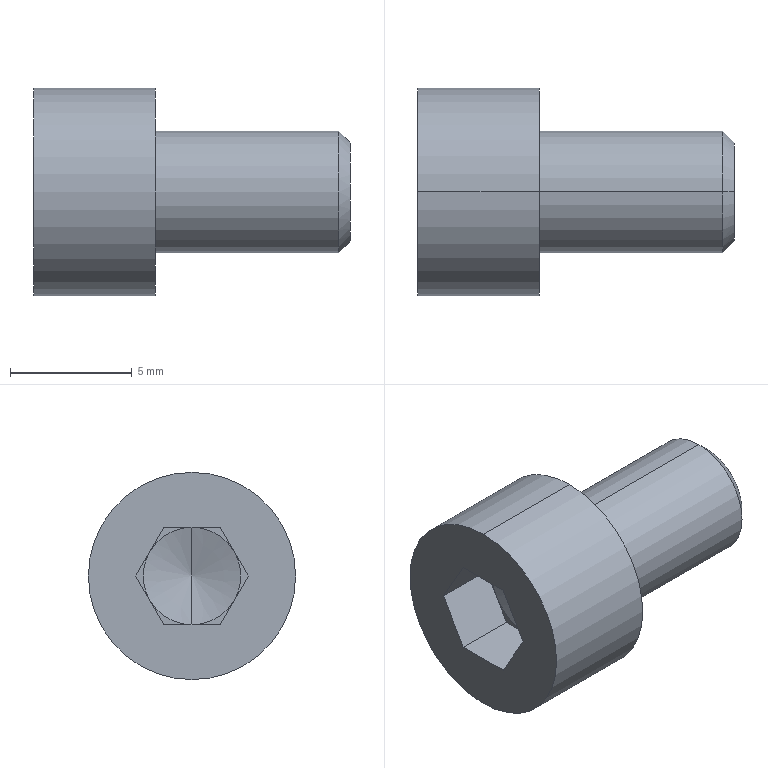Part | SolidWorks | features BaseBody 1 | 1 solid | 23 faces | box 13 x 8.5 x 8.5 mm | volume 402.153 mm3 | plane 15 | cylinder 4 | cone 4 | commonest cylinder face diameters 5 x2 8.5 x2
STEP:
#1=CARTESIAN_POINT('',(-5.,0.,-4.25));
#2=VERTEX_POINT('',#1);
#3=CARTESIAN_POINT('',(-5.,0.,4.25));
#4=VERTEX_POINT('',#3);
#5=CARTESIAN_POINT('',(-5.,0.,0.));
#6=DIRECTION('',(1.,0.,0.));
#7=DIRECTION('',(0.,0.,-1.));
#8=AXIS2_PLACEMENT_3D('',#5,#6,#7);
#9=CIRCLE('',#8,4.25);
#10=EDGE_CURVE('',#2,#4,#9,.T.);
#11=ORIENTED_EDGE('',*,*,#10,.T.);
#12=CARTESIAN_POINT('',(0.,0.,4.25));
#13=VERTEX_POINT('',#12);
#14=CARTESIAN_POINT('',(-2.5,0.,4.25));
#15=DIRECTION('',(1.,0.,0.));
#16=VECTOR('',#15,1000.);
#17=LINE('',#14,#16);
#18=EDGE_CURVE('',#4,#13,#17,.T.);
#19=ORIENTED_EDGE('',*,*,#18,.T.);
#20=CARTESIAN_POINT('',(0.,0.,-4.25));
#21=VERTEX_POINT('',#20);
#22=CARTESIAN_POINT('',(0.,0.,0.));
#23=DIRECTION('',(-1.,0.,0.));
#24=DIRECTION('',(0.,0.,-1.));
#25=AXIS2_PLACEMENT_3D('',#22,#23,#24);
#26=CIRCLE('',#25,4.25);
#27=EDGE_CURVE('',#13,#21,#26,.T.);
#28=ORIENTED_EDGE('',*,*,#27,.T.);
#29=CARTESIAN_POINT('',(-2.5,0.,-4.25));
#30=DIRECTION('',(1.,0.,0.));
#31=VECTOR('',#30,1000.);
#32=LINE('',#29,#31);
#33=EDGE_CURVE('',#2,#21,#32,.T.);
#34=ORIENTED_EDGE('',*,*,#33,.F.);
#35=EDGE_LOOP('',(#11,#19,#28,#34));
#36=FACE_OUTER_BOUND('',#35,.T.);
#37=CARTESIAN_POINT('',(-2.5,0.,0.));
#38=DIRECTION('',(1.,0.,0.));
#39=DIRECTION('',(0.,0.,-1.));
#40=AXIS2_PLACEMENT_3D('',#37,#38,#39);
#41=CYLINDRICAL_SURFACE('',#40,4.25);
#42=ADVANCED_FACE('',(#36),#41,.T.);
#43=CARTESIAN_POINT('',(0.,0.,2.5));
#44=VERTEX_POINT('',#43);
#45=CARTESIAN_POINT('',(0.,0.,-2.5));
#46=VERTEX_POINT('',#45);
#47=CARTESIAN_POINT('',(0.,0.,0.));
#48=DIRECTION('',(-1.,0.,0.));
#49=DIRECTION('',(0.,0.,-1.));
#50=AXIS2_PLACEMENT_3D('',#47,#48,#49);
#51=CIRCLE('',#50,2.5);
#52=EDGE_CURVE('',#44,#46,#51,.T.);
#53=ORIENTED_EDGE('',*,*,#52,.F.);
#54=CARTESIAN_POINT('',(7.51,0.,2.5));
#55=VERTEX_POINT('',#54);
#56=CARTESIAN_POINT('',(3.755,0.,2.5));
#57=DIRECTION('',(1.,0.,0.));
#58=VECTOR('',#57,1000.);
#59=LINE('',#56,#58);
#60=EDGE_CURVE('',#44,#55,#59,.T.);
#61=ORIENTED_EDGE('',*,*,#60,.T.);
#62=CARTESIAN_POINT('',(7.51,0.,-2.5));
#63=VERTEX_POINT('',#62);
#64=CARTESIAN_POINT('',(7.51,0.,0.));
#65=DIRECTION('',(-1.,0.,0.));
#66=DIRECTION('',(0.,0.,-1.));
#67=AXIS2_PLACEMENT_3D('',#64,#65,#66);
#68=CIRCLE('',#67,2.5);
#69=EDGE_CURVE('',#55,#63,#68,.T.);
#70=ORIENTED_EDGE('',*,*,#69,.T.);
#71=CARTESIAN_POINT('',(3.755,0.,-2.5));
#72=DIRECTION('',(1.,0.,0.));
#73=VECTOR('',#72,1000.);
#74=LINE('',#71,#73);
#75=EDGE_CURVE('',#46,#63,#74,.T.);
#76=ORIENTED_EDGE('',*,*,#75,.F.);
#77=EDGE_LOOP('',(#53,#61,#70,#76));
#78=FACE_OUTER_BOUND('',#77,.T.);
#79=CARTESIAN_POINT('',(3.755,0.,0.));
#80=DIRECTION('',(1.,0.,0.));
#81=DIRECTION('',(0.,0.,-1.));
#82=AXIS2_PLACEMENT_3D('',#79,#80,#81);
#83=CYLINDRICAL_SURFACE('',#82,2.5);
#84=ADVANCED_FACE('',(#78),#83,.T.);
#85=CARTESIAN_POINT('',(8.,0.,2.009));
#86=VERTEX_POINT('',#85);
#87=CARTESIAN_POINT('',(8.,0.,-2.009));
#88=VERTEX_POINT('',#87);
#89=CARTESIAN_POINT('',(8.,0.,0.));
#90=DIRECTION('',(-1.,0.,0.));
#91=DIRECTION('',(0.,0.,1.));
#92=AXIS2_PLACEMENT_3D('',#89,#90,#91);
#93=CIRCLE('',#92,2.009);
#94=EDGE_CURVE('',#86,#88,#93,.T.);
#95=ORIENTED_EDGE('',*,*,#94,.T.);
#96=CARTESIAN_POINT('',(7.51,0.,-2.5));
#97=DIRECTION('',(-0.7071,0.,-0.7071));
#98=VECTOR('',#97,1000.);
#99=LINE('',#96,#98);
#100=EDGE_CURVE('',#88,#63,#99,.T.);
#101=ORIENTED_EDGE('',*,*,#100,.T.);
#102=ORIENTED_EDGE('',*,*,#69,.F.);
#103=CARTESIAN_POINT('',(7.51,0.,2.5));
#104=DIRECTION('',(-0.7071,0.,0.7071));
#105=VECTOR('',#104,1000.);
#106=LINE('',#103,#105);
#107=EDGE_CURVE('',#86,#55,#106,.T.);
#108=ORIENTED_EDGE('',*,*,#107,.F.);
#109=EDGE_LOOP('',(#95,#101,#102,#108));
#110=FACE_OUTER_BOUND('',#109,.T.);
#111=CARTESIAN_POINT('',(7.51,0.,0.));
#112=DIRECTION('',(-1.,0.,0.));
#113=DIRECTION('',(0.,0.,1.));
#114=AXIS2_PLACEMENT_3D('',#111,#112,#113);
#115=CONICAL_SURFACE('',#114,2.5,0.7854);
#116=ADVANCED_FACE('',(#110),#115,.T.);
#117=CARTESIAN_POINT('',(-1.964,0.000000001,0.));
#118=VERTEX_POINT('',#117);
#119=CARTESIAN_POINT('',(-2.5,0.,2.));
#120=VERTEX_POINT('',#119);
#121=CARTESIAN_POINT('',(-2.5,0.,2.));
#122=DIRECTION('',(-0.2588,0.,0.9659));
#123=VECTOR('',#122,1000.);
#124=LINE('',#121,#123);
#125=EDGE_CURVE('',#118,#120,#124,.T.);
#126=ORIENTED_EDGE('',*,*,#125,.F.);
#127=CARTESIAN_POINT('',(-2.5,0.,-2.));
#128=VERTEX_POINT('',#127);
#129=CARTESIAN_POINT('',(-2.5,0.,-2.));
#130=DIRECTION('',(-0.2588,0.,-0.9659));
#131=VECTOR('',#130,1000.);
#132=LINE('',#129,#131);
#133=EDGE_CURVE('',#118,#128,#132,.T.);
#134=ORIENTED_EDGE('',*,*,#133,.T.);
#135=CARTESIAN_POINT('',(-2.5,-1.732,-1.));
#136=VERTEX_POINT('',#135);
#137=CARTESIAN_POINT('',(-2.5,0.,0.));
#138=DIRECTION('',(1.,0.,0.));
#139=DIRECTION('',(0.,0.,1.));
#140=AXIS2_PLACEMENT_3D('',#137,#138,#139);
#141=CIRCLE('',#140,2.);
#142=EDGE_CURVE('',#136,#128,#141,.T.);
#143=ORIENTED_EDGE('',*,*,#142,.F.);
#144=CARTESIAN_POINT('',(-2.5,-1.732,1.));
#145=VERTEX_POINT('',#144);
#146=CARTESIAN_POINT('',(-2.5,0.,0.));
#147=DIRECTION('',(1.,0.,0.));
#148=DIRECTION('',(0.,0.,1.));
#149=AXIS2_PLACEMENT_3D('',#146,#147,#148);
#150=CIRCLE('',#149,2.);
#151=EDGE_CURVE('',#145,#136,#150,.T.);
#152=ORIENTED_EDGE('',*,*,#151,.F.);
#153=CARTESIAN_POINT('',(-2.5,0.,0.));
#154=DIRECTION('',(-1.,0.,0.));
#155=DIRECTION('',(0.,0.,1.));
#156=AXIS2_PLACEMENT_3D('',#153,#154,#155);
#157=CIRCLE('',#156,2.);
#158=EDGE_CURVE('',#145,#120,#157,.T.);
#159=ORIENTED_EDGE('',*,*,#158,.T.);
#160=EDGE_LOOP('',(#126,#134,#143,#152,#159));
#161=FACE_OUTER_BOUND('',#160,.T.);
#162=CARTESIAN_POINT('',(-2.5,0.,0.));
#163=DIRECTION('',(-1.,0.,0.));
#164=DIRECTION('',(0.,0.,1.));
#165=AXIS2_PLACEMENT_3D('',#162,#163,#164);
#166=CONICAL_SURFACE('',#165,2.,1.309);
#167=ADVANCED_FACE('',(#161),#166,.F.);
#168=ORIENTED_EDGE('',*,*,#18,.F.);
#169=CARTESIAN_POINT('',(-5.,0.,0.));
#170=DIRECTION('',(1.,0.,0.));
#171=DIRECTION('',(0.,0.,-1.));
#172=AXIS2_PLACEMENT_3D('',#169,#170,#171);
#173=CIRCLE('',#172,4.25);
#174=EDGE_CURVE('',#4,#2,#173,.T.);
#175=ORIENTED_EDGE('',*,*,#174,.T.);
#176=ORIENTED_EDGE('',*,*,#33,.T.);
#177=CARTESIAN_POINT('',(0.,0.,0.));
#178=DIRECTION('',(-1.,0.,0.));
#179=DIRECTION('',(0.,0.,-1.));
#180=AXIS2_PLACEMENT_3D('',#177,#178,#179);
#181=CIRCLE('',#180,4.25);
#182=EDGE_CURVE('',#21,#13,#181,.T.);
#183=ORIENTED_EDGE('',*,*,#182,.T.);
#184=EDGE_LOOP('',(#168,#175,#176,#183));
#185=FACE_OUTER_BOUND('',#184,.T.);
#186=CARTESIAN_POINT('',(-2.5,0.,0.));
#187=DIRECTION('',(1.,0.,0.));
#188=DIRECTION('',(0.,0.,-1.));
#189=AXIS2_PLACEMENT_3D('',#186,#187,#188);
#190=CYLINDRICAL_SURFACE('',#189,4.25);
#191=ADVANCED_FACE('',(#185),#190,.T.);
#192=ORIENTED_EDGE('',*,*,#10,.F.);
#193=ORIENTED_EDGE('',*,*,#174,.F.);
#194=EDGE_LOOP('',(#192,#193));
#195=FACE_OUTER_BOUND('',#194,.T.);
#196=CARTESIAN_POINT('',(-5.,1.155,-2.));
#197=VERTEX_POINT('',#196);
#198=CARTESIAN_POINT('',(-5.,2.309,0.));
#199=VERTEX_POINT('',#198);
#200=CARTESIAN_POINT('',(-5.,1.155,-2.));
#201=DIRECTION('',(0.,0.5,0.866));
#202=VECTOR('',#201,1000.);
#203=LINE('',#200,#202);
#204=EDGE_CURVE('',#197,#199,#203,.T.);
#205=ORIENTED_EDGE('',*,*,#204,.T.);
#206=CARTESIAN_POINT('',(-5.,1.155,2.));
#207=VERTEX_POINT('',#206);
#208=CARTESIAN_POINT('',(-5.,2.309,0.));
#209=DIRECTION('',(0.,-0.5,0.866));
#210=VECTOR('',#209,1000.);
#211=LINE('',#208,#210);
#212=EDGE_CURVE('',#199,#207,#211,.T.);
#213=ORIENTED_EDGE('',*,*,#212,.T.);
#214=CARTESIAN_POINT('',(-5.,-1.155,2.));
#215=VERTEX_POINT('',#214);
#216=CARTESIAN_POINT('',(-5.,2.125,2.));
#217=DIRECTION('',(0.,-1.,0.));
#218=VECTOR('',#217,1000.);
#219=LINE('',#216,#218);
#220=EDGE_CURVE('',#207,#215,#219,.T.);
#221=ORIENTED_EDGE('',*,*,#220,.T.);
#222=CARTESIAN_POINT('',(-5.,-2.309,0.));
#223=VERTEX_POINT('',#222);
#224=CARTESIAN_POINT('',(-5.,-1.155,2.));
#225=DIRECTION('',(0.,-0.5,-0.866));
#226=VECTOR('',#225,1000.);
#227=LINE('',#224,#226);
#228=EDGE_CURVE('',#215,#223,#227,.T.);
#229=ORIENTED_EDGE('',*,*,#228,.T.);
#230=CARTESIAN_POINT('',(-5.,-1.155,-2.));
#231=VERTEX_POINT('',#230);
#232=CARTESIAN_POINT('',(-5.,-2.309,0.));
#233=DIRECTION('',(0.,0.5,-0.866));
#234=VECTOR('',#233,1000.);
#235=LINE('',#232,#234);
#236=EDGE_CURVE('',#223,#231,#235,.T.);
#237=ORIENTED_EDGE('',*,*,#236,.T.);
#238=CARTESIAN_POINT('',(-5.,2.125,-2.));
#239=DIRECTION('',(0.,1.,0.));
#240=VECTOR('',#239,1000.);
#241=LINE('',#238,#240);
#242=EDGE_CURVE('',#231,#197,#241,.T.);
#243=ORIENTED_EDGE('',*,*,#242,.T.);
#244=EDGE_LOOP('',(#205,#213,#221,#229,#237,#243));
#245=FACE_BOUND('',#244,.T.);
#246=CARTESIAN_POINT('',(-5.,2.125,0.));
#247=DIRECTION('',(-1.,0.,0.));
#248=DIRECTION('',(0.,0.,1.));
#249=AXIS2_PLACEMENT_3D('',#246,#247,#248);
#250=PLANE('',#249);
#251=ADVANCED_FACE('',(#195,#245),#250,.T.);
#252=CARTESIAN_POINT('',(0.,0.,0.));
#253=DIRECTION('',(-1.,0.,0.));
#254=DIRECTION('',(0.,0.,-1.));
#255=AXIS2_PLACEMENT_3D('',#252,#253,#254);
#256=CIRCLE('',#255,2.5);
#257=EDGE_CURVE('',#46,#44,#256,.T.);
#258=ORIENTED_EDGE('',*,*,#257,.T.);
#259=ORIENTED_EDGE('',*,*,#52,.T.);
#260=EDGE_LOOP('',(#258,#259));
#261=FACE_BOUND('',#260,.T.);
#262=ORIENTED_EDGE('',*,*,#182,.F.);
#263=ORIENTED_EDGE('',*,*,#27,.F.);
#264=EDGE_LOOP('',(#262,#263));
#265=FACE_OUTER_BOUND('',#264,.T.);
#266=CARTESIAN_POINT('',(0.,3.375,0.));
#267=DIRECTION('',(1.,0.,0.));
#268=DIRECTION('',(0.,0.,-1.));
#269=AXIS2_PLACEMENT_3D('',#266,#267,#268);
#270=PLANE('',#269);
#271=ADVANCED_FACE('',(#261,#265),#270,.T.);
#272=CARTESIAN_POINT('',(-2.5,2.309,0.));
#273=VERTEX_POINT('',#272);
#274=CARTESIAN_POINT('',(-5.,2.309,0.));
#275=DIRECTION('',(-1.,0.,0.));
#276=VECTOR('',#275,1000.);
#277=LINE('',#274,#276);
#278=EDGE_CURVE('',#273,#199,#277,.T.);
#279=ORIENTED_EDGE('',*,*,#278,.F.);
#280=CARTESIAN_POINT('',(-2.5,1.732,1.));
#281=VERTEX_POINT('',#280);
#282=CARTESIAN_POINT('',(-2.5,1.155,2.));
#283=DIRECTION('',(0.,0.5,-0.866));
#284=VECTOR('',#283,1000.);
#285=LINE('',#282,#284);
#286=EDGE_CURVE('',#281,#273,#285,.T.);
#287=ORIENTED_EDGE('',*,*,#286,.F.);
#288=CARTESIAN_POINT('',(-2.5,1.155,2.));
#289=VERTEX_POINT('',#288);
#290=CARTESIAN_POINT('',(-2.5,1.732,1.));
#291=DIRECTION('',(0.,-0.5,0.866));
#292=VECTOR('',#291,1000.);
#293=LINE('',#290,#292);
#294=EDGE_CURVE('',#281,#289,#293,.T.);
#295=ORIENTED_EDGE('',*,*,#294,.T.);
#296=CARTESIAN_POINT('',(-5.,1.155,2.));
#297=DIRECTION('',(1.,0.,0.));
#298=VECTOR('',#297,1000.);
#299=LINE('',#296,#298);
#300=EDGE_CURVE('',#207,#289,#299,.T.);
#301=ORIENTED_EDGE('',*,*,#300,.F.);
#302=ORIENTED_EDGE('',*,*,#212,.F.);
#303=EDGE_LOOP('',(#279,#287,#295,#301,#302));
#304=FACE_OUTER_BOUND('',#303,.T.);
#305=CARTESIAN_POINT('',(-5.,1.155,2.));
#306=DIRECTION('',(0.,0.866,0.5));
#307=DIRECTION('',(0.,-0.5,0.866));
#308=AXIS2_PLACEMENT_3D('',#305,#306,#307);
#309=PLANE('',#308);
#310=ADVANCED_FACE('',(#304),#309,.F.);
#311=CARTESIAN_POINT('',(-2.5,1.155,-2.));
#312=VERTEX_POINT('',#311);
#313=CARTESIAN_POINT('',(-5.,1.155,-2.));
#314=DIRECTION('',(-1.,0.,0.));
#315=VECTOR('',#314,1000.);
#316=LINE('',#313,#315);
#317=EDGE_CURVE('',#312,#197,#316,.T.);
#318=ORIENTED_EDGE('',*,*,#317,.F.);
#319=CARTESIAN_POINT('',(-2.5,1.732,-1.));
#320=VERTEX_POINT('',#319);
#321=CARTESIAN_POINT('',(-2.5,1.155,-2.));
#322=DIRECTION('',(0.,0.5,0.866));
#323=VECTOR('',#322,1000.);
#324=LINE('',#321,#323);
#325=EDGE_CURVE('',#312,#320,#324,.T.);
#326=ORIENTED_EDGE('',*,*,#325,.T.);
#327=CARTESIAN_POINT('',(-2.5,2.309,0.));
#328=DIRECTION('',(0.,-0.5,-0.866));
#329=VECTOR('',#328,1000.);
#330=LINE('',#327,#329);
#331=EDGE_CURVE('',#273,#320,#330,.T.);
#332=ORIENTED_EDGE('',*,*,#331,.F.);
#333=ORIENTED_EDGE('',*,*,#278,.T.);
#334=ORIENTED_EDGE('',*,*,#204,.F.);
#335=EDGE_LOOP('',(#318,#326,#332,#333,#334));
#336=FACE_OUTER_BOUND('',#335,.T.);
#337=CARTESIAN_POINT('',(-5.,2.309,0.));
#338=DIRECTION('',(0.,0.866,-0.5));
#339=DIRECTION('',(0.,0.5,0.866));
#340=AXIS2_PLACEMENT_3D('',#337,#338,#339);
#341=PLANE('',#340);
#342=ADVANCED_FACE('',(#336),#341,.F.);
#343=CARTESIAN_POINT('',(-2.5,-1.155,-2.));
#344=VERTEX_POINT('',#343);
#345=CARTESIAN_POINT('',(-5.,-1.155,-2.));
#346=DIRECTION('',(-1.,0.,0.));
#347=VECTOR('',#346,1000.);
#348=LINE('',#345,#347);
#349=EDGE_CURVE('',#344,#231,#348,.T.);
#350=ORIENTED_EDGE('',*,*,#349,.F.);
#351=CARTESIAN_POINT('',(-2.5,0.,-2.));
#352=DIRECTION('',(0.,1.,0.));
#353=VECTOR('',#352,1000.);
#354=LINE('',#351,#353);
#355=EDGE_CURVE('',#344,#128,#354,.T.);
#356=ORIENTED_EDGE('',*,*,#355,.T.);
#357=CARTESIAN_POINT('',(-2.5,0.,-2.));
#358=DIRECTION('',(0.,1.,0.));
#359=VECTOR('',#358,1000.);
#360=LINE('',#357,#359);
#361=EDGE_CURVE('',#128,#312,#360,.T.);
#362=ORIENTED_EDGE('',*,*,#361,.T.);
#363=ORIENTED_EDGE('',*,*,#317,.T.);
#364=ORIENTED_EDGE('',*,*,#242,.F.);
#365=EDGE_LOOP('',(#350,#356,#362,#363,#364));
#366=FACE_OUTER_BOUND('',#365,.T.);
#367=CARTESIAN_POINT('',(-5.,1.155,-2.));
#368=DIRECTION('',(0.,0.,-1.));
#369=DIRECTION('',(-1.,0.,0.));
#370=AXIS2_PLACEMENT_3D('',#367,#368,#369);
#371=PLANE('',#370);
#372=ADVANCED_FACE('',(#366),#371,.F.);
#373=CARTESIAN_POINT('',(-2.5,-2.309,0.));
#374=VERTEX_POINT('',#373);
#375=CARTESIAN_POINT('',(-5.,-2.309,0.));
#376=DIRECTION('',(-1.,0.,0.));
#377=VECTOR('',#376,1000.);
#378=LINE('',#375,#377);
#379=EDGE_CURVE('',#374,#223,#378,.T.);
#380=ORIENTED_EDGE('',*,*,#379,.F.);
#381=CARTESIAN_POINT('',(-2.5,-1.155,-2.));
#382=DIRECTION('',(0.,-0.5,0.866));
#383=VECTOR('',#382,1000.);
#384=LINE('',#381,#383);
#385=EDGE_CURVE('',#136,#374,#384,.T.);
#386=ORIENTED_EDGE('',*,*,#385,.F.);
#387=CARTESIAN_POINT('',(-2.5,-1.732,-1.));
#388=DIRECTION('',(0.,0.5,-0.866));
#389=VECTOR('',#388,1000.);
#390=LINE('',#387,#389);
#391=EDGE_CURVE('',#136,#344,#390,.T.);
#392=ORIENTED_EDGE('',*,*,#391,.T.);
#393=ORIENTED_EDGE('',*,*,#349,.T.);
#394=ORIENTED_EDGE('',*,*,#236,.F.);
#395=EDGE_LOOP('',(#380,#386,#392,#393,#394));
#396=FACE_OUTER_BOUND('',#395,.T.);
#397=CARTESIAN_POINT('',(-5.,-1.155,-2.));
#398=DIRECTION('',(0.,-0.866,-0.5));
#399=DIRECTION('',(0.,0.5,-0.866));
#400=AXIS2_PLACEMENT_3D('',#397,#398,#399);
#401=PLANE('',#400);
#402=ADVANCED_FACE('',(#396),#401,.F.);
#403=CARTESIAN_POINT('',(-2.5,-1.155,2.));
#404=VERTEX_POINT('',#403);
#405=CARTESIAN_POINT('',(-5.,-1.155,2.));
#406=DIRECTION('',(-1.,0.,0.));
#407=VECTOR('',#406,1000.);
#408=LINE('',#405,#407);
#409=EDGE_CURVE('',#404,#215,#408,.T.);
#410=ORIENTED_EDGE('',*,*,#409,.F.);
#411=CARTESIAN_POINT('',(-2.5,-2.309,0.));
#412=DIRECTION('',(0.,0.5,0.866));
#413=VECTOR('',#412,1000.);
#414=LINE('',#411,#413);
#415=EDGE_CURVE('',#145,#404,#414,.T.);
#416=ORIENTED_EDGE('',*,*,#415,.F.);
#417=CARTESIAN_POINT('',(-2.5,-2.309,0.));
#418=DIRECTION('',(0.,0.5,0.866));
#419=VECTOR('',#418,1000.);
#420=LINE('',#417,#419);
#421=EDGE_CURVE('',#374,#145,#420,.T.);
#422=ORIENTED_EDGE('',*,*,#421,.F.);
#423=ORIENTED_EDGE('',*,*,#379,.T.);
#424=ORIENTED_EDGE('',*,*,#228,.F.);
#425=EDGE_LOOP('',(#410,#416,#422,#423,#424));
#426=FACE_OUTER_BOUND('',#425,.T.);
#427=CARTESIAN_POINT('',(-5.,-2.309,0.));
#428=DIRECTION('',(0.,-0.866,0.5));
#429=DIRECTION('',(0.,-0.5,-0.866));
#430=AXIS2_PLACEMENT_3D('',#427,#428,#429);
#431=PLANE('',#430);
#432=ADVANCED_FACE('',(#426),#431,.F.);
#433=ORIENTED_EDGE('',*,*,#300,.T.);
#434=CARTESIAN_POINT('',(-2.5,0.,2.));
#435=DIRECTION('',(0.,-1.,0.));
#436=VECTOR('',#435,1000.);
#437=LINE('',#434,#436);
#438=EDGE_CURVE('',#289,#120,#437,.T.);
#439=ORIENTED_EDGE('',*,*,#438,.T.);
#440=CARTESIAN_POINT('',(-2.5,-1.155,2.));
#441=DIRECTION('',(0.,1.,0.));
#442=VECTOR('',#441,1000.);
#443=LINE('',#440,#442);
#444=EDGE_CURVE('',#404,#120,#443,.T.);
#445=ORIENTED_EDGE('',*,*,#444,.F.);
#446=ORIENTED_EDGE('',*,*,#409,.T.);
#447=ORIENTED_EDGE('',*,*,#220,.F.);
#448=EDGE_LOOP('',(#433,#439,#445,#446,#447));
#449=FACE_OUTER_BOUND('',#448,.T.);
#450=CARTESIAN_POINT('',(-5.,-1.155,2.));
#451=DIRECTION('',(0.,0.,1.));
#452=DIRECTION('',(1.,0.,0.));
#453=AXIS2_PLACEMENT_3D('',#450,#451,#452);
#454=PLANE('',#453);
#455=ADVANCED_FACE('',(#449),#454,.F.);
#456=ORIENTED_EDGE('',*,*,#60,.F.);
#457=ORIENTED_EDGE('',*,*,#257,.F.);
#458=ORIENTED_EDGE('',*,*,#75,.T.);
#459=CARTESIAN_POINT('',(7.51,0.,0.));
#460=DIRECTION('',(-1.,0.,0.));
#461=DIRECTION('',(0.,0.,-1.));
#462=AXIS2_PLACEMENT_3D('',#459,#460,#461);
#463=CIRCLE('',#462,2.5);
#464=EDGE_CURVE('',#63,#55,#463,.T.);
#465=ORIENTED_EDGE('',*,*,#464,.T.);
#466=EDGE_LOOP('',(#456,#457,#458,#465));
#467=FACE_OUTER_BOUND('',#466,.T.);
#468=CARTESIAN_POINT('',(3.755,0.,0.));
#469=DIRECTION('',(1.,0.,0.));
#470=DIRECTION('',(0.,0.,-1.));
#471=AXIS2_PLACEMENT_3D('',#468,#469,#470);
#472=CYLINDRICAL_SURFACE('',#471,2.5);
#473=ADVANCED_FACE('',(#467),#472,.T.);
#474=ORIENTED_EDGE('',*,*,#286,.T.);
#475=ORIENTED_EDGE('',*,*,#331,.T.);
#476=CARTESIAN_POINT('',(-2.5,0.,0.));
#477=DIRECTION('',(1.,0.,0.));
#478=DIRECTION('',(0.,0.,1.));
#479=AXIS2_PLACEMENT_3D('',#476,#477,#478);
#480=CIRCLE('',#479,2.);
#481=EDGE_CURVE('',#320,#281,#480,.T.);
#482=ORIENTED_EDGE('',*,*,#481,.T.);
#483=EDGE_LOOP('',(#474,#475,#482));
#484=FACE_OUTER_BOUND('',#483,.T.);
#485=CARTESIAN_POINT('',(-2.5,0.,0.));
#486=DIRECTION('',(1.,0.,0.));
#487=DIRECTION('',(0.,0.,-1.));
#488=AXIS2_PLACEMENT_3D('',#485,#486,#487);
#489=PLANE('',#488);
#490=ADVANCED_FACE('',(#484),#489,.F.);
#491=ORIENTED_EDGE('',*,*,#385,.T.);
#492=ORIENTED_EDGE('',*,*,#421,.T.);
#493=ORIENTED_EDGE('',*,*,#151,.T.);
#494=EDGE_LOOP('',(#491,#492,#493));
#495=FACE_OUTER_BOUND('',#494,.T.);
#496=CARTESIAN_POINT('',(-2.5,0.,0.));
#497=DIRECTION('',(1.,0.,0.));
#498=DIRECTION('',(0.,0.,-1.));
#499=AXIS2_PLACEMENT_3D('',#496,#497,#498);
#500=PLANE('',#499);
#501=ADVANCED_FACE('',(#495),#500,.F.);
#502=ORIENTED_EDGE('',*,*,#415,.T.);
#503=ORIENTED_EDGE('',*,*,#444,.T.);
#504=ORIENTED_EDGE('',*,*,#158,.F.);
#505=EDGE_LOOP('',(#502,#503,#504));
#506=FACE_OUTER_BOUND('',#505,.T.);
#507=CARTESIAN_POINT('',(-2.5,0.,0.));
#508=DIRECTION('',(1.,0.,0.));
#509=DIRECTION('',(0.,0.,-1.));
#510=AXIS2_PLACEMENT_3D('',#507,#508,#509);
#511=PLANE('',#510);
#512=ADVANCED_FACE('',(#506),#511,.F.);
#513=ORIENTED_EDGE('',*,*,#100,.F.);
#514=CARTESIAN_POINT('',(8.,0.,0.));
#515=DIRECTION('',(-1.,0.,0.));
#516=DIRECTION('',(0.,0.,1.));
#517=AXIS2_PLACEMENT_3D('',#514,#515,#516);
#518=CIRCLE('',#517,2.009);
#519=EDGE_CURVE('',#88,#86,#518,.T.);
#520=ORIENTED_EDGE('',*,*,#519,.T.);
#521=ORIENTED_EDGE('',*,*,#107,.T.);
#522=ORIENTED_EDGE('',*,*,#464,.F.);
#523=EDGE_LOOP('',(#513,#520,#521,#522));
#524=FACE_OUTER_BOUND('',#523,.T.);
#525=CARTESIAN_POINT('',(7.51,0.,0.));
#526=DIRECTION('',(-1.,0.,0.));
#527=DIRECTION('',(0.,0.,1.));
#528=AXIS2_PLACEMENT_3D('',#525,#526,#527);
#529=CONICAL_SURFACE('',#528,2.5,0.7854);
#530=ADVANCED_FACE('',(#524),#529,.T.);
#531=ORIENTED_EDGE('',*,*,#133,.F.);
#532=ORIENTED_EDGE('',*,*,#125,.T.);
#533=CARTESIAN_POINT('',(-2.5,0.,0.));
#534=DIRECTION('',(1.,0.,0.));
#535=DIRECTION('',(0.,0.,1.));
#536=AXIS2_PLACEMENT_3D('',#533,#534,#535);
#537=CIRCLE('',#536,2.);
#538=EDGE_CURVE('',#281,#120,#537,.T.);
#539=ORIENTED_EDGE('',*,*,#538,.F.);
#540=ORIENTED_EDGE('',*,*,#481,.F.);
#541=CARTESIAN_POINT('',(-2.5,0.,0.));
#542=DIRECTION('',(1.,0.,0.));
#543=DIRECTION('',(0.,0.,1.));
#544=AXIS2_PLACEMENT_3D('',#541,#542,#543);
#545=CIRCLE('',#544,2.);
#546=EDGE_CURVE('',#128,#320,#545,.T.);
#547=ORIENTED_EDGE('',*,*,#546,.F.);
#548=EDGE_LOOP('',(#531,#532,#539,#540,#547));
#549=FACE_OUTER_BOUND('',#548,.T.);
#550=CARTESIAN_POINT('',(-2.5,0.,0.));
#551=DIRECTION('',(-1.,0.,0.));
#552=DIRECTION('',(0.,0.,1.));
#553=AXIS2_PLACEMENT_3D('',#550,#551,#552);
#554=CONICAL_SURFACE('',#553,2.,1.309);
#555=ADVANCED_FACE('',(#549),#554,.F.);
#556=ORIENTED_EDGE('',*,*,#94,.F.);
#557=ORIENTED_EDGE('',*,*,#519,.F.);
#558=EDGE_LOOP('',(#556,#557));
#559=FACE_OUTER_BOUND('',#558,.T.);
#560=CARTESIAN_POINT('',(8.,1.005,0.));
#561=DIRECTION('',(1.,0.,0.));
#562=DIRECTION('',(0.,0.,-1.));
#563=AXIS2_PLACEMENT_3D('',#560,#561,#562);
#564=PLANE('',#563);
#565=ADVANCED_FACE('',(#559),#564,.T.);
#566=ORIENTED_EDGE('',*,*,#438,.F.);
#567=ORIENTED_EDGE('',*,*,#294,.F.);
#568=ORIENTED_EDGE('',*,*,#538,.T.);
#569=EDGE_LOOP('',(#566,#567,#568));
#570=FACE_OUTER_BOUND('',#569,.T.);
#571=CARTESIAN_POINT('',(-2.5,0.,0.));
#572=DIRECTION('',(1.,0.,0.));
#573=DIRECTION('',(0.,0.,-1.));
#574=AXIS2_PLACEMENT_3D('',#571,#572,#573);
#575=PLANE('',#574);
#576=ADVANCED_FACE('',(#570),#575,.F.);
#577=ORIENTED_EDGE('',*,*,#325,.F.);
#578=ORIENTED_EDGE('',*,*,#361,.F.);
#579=ORIENTED_EDGE('',*,*,#546,.T.);
#580=EDGE_LOOP('',(#577,#578,#579));
#581=FACE_OUTER_BOUND('',#580,.T.);
#582=CARTESIAN_POINT('',(-2.5,0.,0.));
#583=DIRECTION('',(1.,0.,0.));
#584=DIRECTION('',(0.,0.,-1.));
#585=AXIS2_PLACEMENT_3D('',#582,#583,#584);
#586=PLANE('',#585);
#587=ADVANCED_FACE('',(#581),#586,.F.);
#588=ORIENTED_EDGE('',*,*,#355,.F.);
#589=ORIENTED_EDGE('',*,*,#391,.F.);
#590=ORIENTED_EDGE('',*,*,#142,.T.);
#591=EDGE_LOOP('',(#588,#589,#590));
#592=FACE_OUTER_BOUND('',#591,.T.);
#593=CARTESIAN_POINT('',(-2.5,0.,0.));
#594=DIRECTION('',(1.,0.,0.));
#595=DIRECTION('',(0.,0.,-1.));
#596=AXIS2_PLACEMENT_3D('',#593,#594,#595);
#597=PLANE('',#596);
#598=ADVANCED_FACE('',(#592),#597,.F.);
#599=CLOSED_SHELL('',(#42,#84,#116,#167,#191,#251,#271,#310,#342,#372,#402,#432,#455,#473,#490,#501,#512,#530,#555,#565,#576,#587,#598));
#600=MANIFOLD_SOLID_BREP('',#599);
#601=CARTESIAN_POINT('',(0.,0.,0.));
#602=DIRECTION('',(0.,0.,1.));
#603=DIRECTION('',(1.,0.,0.));
#604=AXIS2_PLACEMENT_3D('',#601,#602,#603);
#605=(LENGTH_UNIT()NAMED_UNIT(*)SI_UNIT(.MILLI.,.METRE.));
#606=UNCERTAINTY_MEASURE_WITH_UNIT(LENGTH_MEASURE(0.00001),#605,'','');
#607=(NAMED_UNIT(*)PLANE_ANGLE_UNIT()SI_UNIT($,.RADIAN.));
#608=(NAMED_UNIT(*)SI_UNIT($,.STERADIAN.)SOLID_ANGLE_UNIT());
#609=(GEOMETRIC_REPRESENTATION_CONTEXT(3)GLOBAL_UNCERTAINTY_ASSIGNED_CONTEXT((#606))GLOBAL_UNIT_ASSIGNED_CONTEXT((#605,#607,#608))REPRESENTATION_CONTEXT('',''));
#610=ADVANCED_BREP_SHAPE_REPRESENTATION('',(#600,#604),#609);